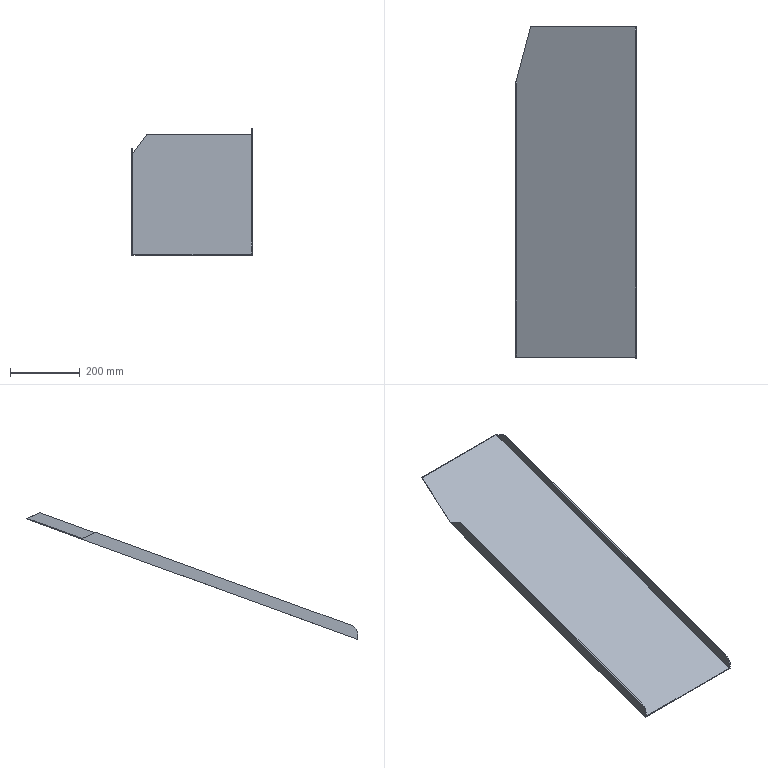Part | NX | features solid 2 | 1 solid | 14 faces | box 344.217 x 951.809 x 363.702 mm | volume 792307 mm3 | plane 12 | cylinder 2 | commonest cylinder face diameters 60 x2
STEP:
#1=CARTESIAN_POINT('',(718.,-1180.,-590.79));
#2=VERTEX_POINT('',#1);
#3=CARTESIAN_POINT('',(375.783,-1180.,-590.79));
#4=VERTEX_POINT('',#3);
#5=CARTESIAN_POINT('',(-625.,-1180.,-590.79));
#6=DIRECTION('',(1.,0.,0.));
#7=VECTOR('',#6,1000.);
#8=LINE('',#5,#7);
#9=EDGE_CURVE('',#2,#4,#8,.F.);
#10=ORIENTED_EDGE('',*,*,#9,.F.);
#11=CARTESIAN_POINT('',(718.,-1180.,-588.662));
#12=VERTEX_POINT('',#11);
#13=CARTESIAN_POINT('',(718.,-1180.,-730.));
#14=DIRECTION('',(0.,0.,-1.));
#15=VECTOR('',#14,1000.);
#16=LINE('',#13,#15);
#17=EDGE_CURVE('',#2,#12,#16,.F.);
#18=ORIENTED_EDGE('',*,*,#17,.T.);
#19=CARTESIAN_POINT('',(377.783,-1180.,-588.662));
#20=VERTEX_POINT('',#19);
#21=CARTESIAN_POINT('',(-625.,-1180.,-588.662));
#22=DIRECTION('',(1.,0.,0.));
#23=VECTOR('',#22,1000.);
#24=LINE('',#21,#23);
#25=EDGE_CURVE('',#12,#20,#24,.F.);
#26=ORIENTED_EDGE('',*,*,#25,.T.);
#27=CARTESIAN_POINT('',(375.783,-1180.,-588.662));
#28=VERTEX_POINT('',#27);
#29=CARTESIAN_POINT('',(375.783,-1180.,-588.662));
#30=DIRECTION('',(1.,0.,0.));
#31=VECTOR('',#30,1000.);
#32=LINE('',#29,#31);
#33=EDGE_CURVE('',#28,#20,#32,.T.);
#34=ORIENTED_EDGE('',*,*,#33,.F.);
#35=CARTESIAN_POINT('',(375.783,-1180.,-730.));
#36=DIRECTION('',(0.,0.,1.));
#37=VECTOR('',#36,1000.);
#38=LINE('',#35,#37);
#39=EDGE_CURVE('',#28,#4,#38,.F.);
#40=ORIENTED_EDGE('',*,*,#39,.T.);
#41=EDGE_LOOP('',(#10,#18,#26,#34,#40));
#42=FACE_BOUND('',#41,.T.);
#43=CARTESIAN_POINT('',(-625.,-1180.,-730.));
#44=DIRECTION('',(0.,1.,0.));
#45=DIRECTION('',(1.,0.,0.));
#46=AXIS2_PLACEMENT_3D('',#43,#44,#45);
#47=PLANE('',#46);
#48=ADVANCED_FACE('',(#42),#47,.F.);
#49=CARTESIAN_POINT('',(718.,-232.563,-243.823));
#50=VERTEX_POINT('',#49);
#51=CARTESIAN_POINT('',(718.,-1653.904,-761.149));
#52=DIRECTION('',(0.,0.9397,0.342));
#53=VECTOR('',#52,1000.);
#54=LINE('',#51,#53);
#55=EDGE_CURVE('',#12,#50,#54,.T.);
#56=ORIENTED_EDGE('',*,*,#55,.T.);
#57=CARTESIAN_POINT('',(418.101,-232.563,-243.823));
#58=VERTEX_POINT('',#57);
#59=CARTESIAN_POINT('',(620.,-232.563,-243.823));
#60=DIRECTION('',(-1.,0.,0.));
#61=VECTOR('',#60,1000.);
#62=LINE('',#59,#61);
#63=EDGE_CURVE('',#50,#58,#62,.T.);
#64=ORIENTED_EDGE('',*,*,#63,.T.);
#65=CARTESIAN_POINT('',(375.783,-390.494,-301.305));
#66=VERTEX_POINT('',#65);
#67=CARTESIAN_POINT('',(71.996,-1524.243,-713.956));
#68=DIRECTION('',(-0.2442,-0.9113,-0.3317));
#69=VECTOR('',#68,1000.);
#70=LINE('',#67,#69);
#71=EDGE_CURVE('',#58,#66,#70,.T.);
#72=ORIENTED_EDGE('',*,*,#71,.T.);
#73=CARTESIAN_POINT('',(377.783,-390.494,-301.305));
#74=VERTEX_POINT('',#73);
#75=CARTESIAN_POINT('',(375.783,-390.494,-301.305));
#76=DIRECTION('',(1.,0.,0.));
#77=VECTOR('',#76,1000.);
#78=LINE('',#75,#77);
#79=EDGE_CURVE('',#66,#74,#78,.T.);
#80=ORIENTED_EDGE('',*,*,#79,.T.);
#81=CARTESIAN_POINT('',(377.783,-1180.,-588.662));
#82=DIRECTION('',(0.,0.9397,0.342));
#83=VECTOR('',#82,1000.);
#84=LINE('',#81,#83);
#85=EDGE_CURVE('',#20,#74,#84,.T.);
#86=ORIENTED_EDGE('',*,*,#85,.F.);
#87=ORIENTED_EDGE('',*,*,#25,.F.);
#88=EDGE_LOOP('',(#56,#64,#72,#80,#86,#87));
#89=FACE_BOUND('',#88,.T.);
#90=CARTESIAN_POINT('',(620.,-1653.904,-761.149));
#91=DIRECTION('',(0.,-0.342,0.9397));
#92=DIRECTION('',(1.,0.,0.));
#93=AXIS2_PLACEMENT_3D('',#90,#91,#92);
#94=PLANE('',#93);
#95=ADVANCED_FACE('',(#89),#94,.T.);
#96=ORIENTED_EDGE('',*,*,#71,.F.);
#97=CARTESIAN_POINT('',(418.604,-230.,-245.018));
#98=VERTEX_POINT('',#97);
#99=CARTESIAN_POINT('',(420.543,-220.131,-249.621));
#100=DIRECTION('',(0.1753,0.8923,-0.4161));
#101=VECTOR('',#100,1000.);
#102=LINE('',#99,#101);
#103=EDGE_CURVE('',#58,#98,#102,.T.);
#104=ORIENTED_EDGE('',*,*,#103,.T.);
#105=CARTESIAN_POINT('',(375.783,-389.81,-303.185));
#106=VERTEX_POINT('',#105);
#107=CARTESIAN_POINT('',(71.996,-1523.559,-715.835));
#108=DIRECTION('',(-0.2442,-0.9113,-0.3317));
#109=VECTOR('',#108,1000.);
#110=LINE('',#107,#109);
#111=EDGE_CURVE('',#98,#106,#110,.T.);
#112=ORIENTED_EDGE('',*,*,#111,.T.);
#113=CARTESIAN_POINT('',(375.783,-390.494,-301.305));
#114=DIRECTION('',(0.,0.342,-0.9397));
#115=VECTOR('',#114,1000.);
#116=LINE('',#113,#115);
#117=EDGE_CURVE('',#66,#106,#116,.T.);
#118=ORIENTED_EDGE('',*,*,#117,.F.);
#119=EDGE_LOOP('',(#96,#104,#112,#118));
#120=FACE_BOUND('',#119,.T.);
#121=CARTESIAN_POINT('',(71.996,-1524.243,-713.956));
#122=DIRECTION('',(0.9697,-0.2294,-0.08351));
#123=DIRECTION('',(0.2302,0.9731,0.));
#124=AXIS2_PLACEMENT_3D('',#121,#122,#123);
#125=PLANE('',#124);
#126=ADVANCED_FACE('',(#120),#125,.F.);
#127=CARTESIAN_POINT('',(375.783,-1162.07,-550.21));
#128=VERTEX_POINT('',#127);
#129=CARTESIAN_POINT('',(375.783,-428.946,-283.375));
#130=VERTEX_POINT('',#129);
#131=CARTESIAN_POINT('',(375.783,-1190.261,-560.471));
#132=DIRECTION('',(0.,0.9397,0.342));
#133=VECTOR('',#132,1000.);
#134=LINE('',#131,#133);
#135=EDGE_CURVE('',#128,#130,#134,.T.);
#136=ORIENTED_EDGE('',*,*,#135,.T.);
#137=CARTESIAN_POINT('',(375.783,-1252.121,100.478));
#138=DIRECTION('',(0.,0.9063,-0.4226));
#139=VECTOR('',#138,1000.);
#140=LINE('',#137,#139);
#141=EDGE_CURVE('',#130,#66,#140,.T.);
#142=ORIENTED_EDGE('',*,*,#141,.T.);
#143=ORIENTED_EDGE('',*,*,#117,.T.);
#144=CARTESIAN_POINT('',(375.783,-1653.22,-763.028));
#145=DIRECTION('',(0.,0.9397,0.342));
#146=VECTOR('',#145,1000.);
#147=LINE('',#144,#146);
#148=EDGE_CURVE('',#4,#106,#147,.T.);
#149=ORIENTED_EDGE('',*,*,#148,.F.);
#150=ORIENTED_EDGE('',*,*,#39,.F.);
#151=CARTESIAN_POINT('',(375.783,-1151.809,-578.401));
#152=DIRECTION('',(1.,0.,0.));
#153=DIRECTION('',(0.,1.,0.));
#154=AXIS2_PLACEMENT_3D('',#151,#152,#153);
#155=CIRCLE('',#154,30.);
#156=EDGE_CURVE('',#28,#128,#155,.F.);
#157=ORIENTED_EDGE('',*,*,#156,.T.);
#158=EDGE_LOOP('',(#136,#142,#143,#149,#150,#157));
#159=FACE_BOUND('',#158,.T.);
#160=CARTESIAN_POINT('',(375.783,-1653.904,-761.149));
#161=DIRECTION('',(-1.,0.,0.));
#162=DIRECTION('',(0.,-1.,0.));
#163=AXIS2_PLACEMENT_3D('',#160,#161,#162);
#164=PLANE('',#163);
#165=ADVANCED_FACE('',(#159),#164,.T.);
#166=CARTESIAN_POINT('',(720.,-1180.,-590.79));
#167=VERTEX_POINT('',#166);
#168=CARTESIAN_POINT('',(720.,-230.,-245.018));
#169=VERTEX_POINT('',#168);
#170=CARTESIAN_POINT('',(720.,-1653.22,-763.028));
#171=DIRECTION('',(0.,0.9397,0.342));
#172=VECTOR('',#171,1000.);
#173=LINE('',#170,#172);
#174=EDGE_CURVE('',#167,#169,#173,.T.);
#175=ORIENTED_EDGE('',*,*,#174,.T.);
#176=CARTESIAN_POINT('',(720.,-268.451,-227.088));
#177=VERTEX_POINT('',#176);
#178=CARTESIAN_POINT('',(720.,-268.451,-227.088));
#179=DIRECTION('',(0.,-0.9063,0.4226));
#180=VECTOR('',#179,1000.);
#181=LINE('',#178,#180);
#182=EDGE_CURVE('',#169,#177,#181,.T.);
#183=ORIENTED_EDGE('',*,*,#182,.T.);
#184=CARTESIAN_POINT('',(720.,-1162.07,-552.339));
#185=VERTEX_POINT('',#184);
#186=CARTESIAN_POINT('',(720.,-1190.261,-562.599));
#187=DIRECTION('',(0.,0.9397,0.342));
#188=VECTOR('',#187,1000.);
#189=LINE('',#186,#188);
#190=EDGE_CURVE('',#185,#177,#189,.T.);
#191=ORIENTED_EDGE('',*,*,#190,.F.);
#192=CARTESIAN_POINT('',(720.,-1151.809,-580.529));
#193=DIRECTION('',(1.,0.,0.));
#194=DIRECTION('',(0.,0.,-1.));
#195=AXIS2_PLACEMENT_3D('',#192,#193,#194);
#196=CIRCLE('',#195,30.);
#197=EDGE_CURVE('',#185,#167,#196,.T.);
#198=ORIENTED_EDGE('',*,*,#197,.T.);
#199=EDGE_LOOP('',(#175,#183,#191,#198));
#200=FACE_BOUND('',#199,.T.);
#201=CARTESIAN_POINT('',(720.,-1653.904,-761.149));
#202=DIRECTION('',(-1.,0.,0.));
#203=DIRECTION('',(0.,0.,1.));
#204=AXIS2_PLACEMENT_3D('',#201,#202,#203);
#205=PLANE('',#204);
#206=ADVANCED_FACE('',(#200),#205,.F.);
#207=CARTESIAN_POINT('',(-625.,-1180.,-590.79));
#208=DIRECTION('',(1.,0.,0.));
#209=VECTOR('',#208,1000.);
#210=LINE('',#207,#209);
#211=EDGE_CURVE('',#167,#2,#210,.F.);
#212=ORIENTED_EDGE('',*,*,#211,.T.);
#213=ORIENTED_EDGE('',*,*,#9,.T.);
#214=ORIENTED_EDGE('',*,*,#148,.T.);
#215=ORIENTED_EDGE('',*,*,#111,.F.);
#216=CARTESIAN_POINT('',(620.,-230.,-245.018));
#217=DIRECTION('',(1.,0.,0.));
#218=VECTOR('',#217,1000.);
#219=LINE('',#216,#218);
#220=EDGE_CURVE('',#98,#169,#219,.T.);
#221=ORIENTED_EDGE('',*,*,#220,.T.);
#222=ORIENTED_EDGE('',*,*,#174,.F.);
#223=EDGE_LOOP('',(#212,#213,#214,#215,#221,#222));
#224=FACE_BOUND('',#223,.T.);
#225=CARTESIAN_POINT('',(620.,-1653.22,-763.028));
#226=DIRECTION('',(0.,-0.342,0.9397));
#227=DIRECTION('',(1.,0.,0.));
#228=AXIS2_PLACEMENT_3D('',#225,#226,#227);
#229=PLANE('',#228);
#230=ADVANCED_FACE('',(#224),#229,.F.);
#231=ORIENTED_EDGE('',*,*,#190,.T.);
#232=CARTESIAN_POINT('',(718.,-268.451,-227.088));
#233=VERTEX_POINT('',#232);
#234=CARTESIAN_POINT('',(718.,-268.451,-227.088));
#235=DIRECTION('',(-1.,0.,0.));
#236=VECTOR('',#235,1000.);
#237=LINE('',#234,#236);
#238=EDGE_CURVE('',#177,#233,#237,.T.);
#239=ORIENTED_EDGE('',*,*,#238,.T.);
#240=CARTESIAN_POINT('',(718.,-1162.07,-552.339));
#241=VERTEX_POINT('',#240);
#242=CARTESIAN_POINT('',(718.,-1190.261,-562.599));
#243=DIRECTION('',(0.,0.9397,0.342));
#244=VECTOR('',#243,1000.);
#245=LINE('',#242,#244);
#246=EDGE_CURVE('',#241,#233,#245,.T.);
#247=ORIENTED_EDGE('',*,*,#246,.F.);
#248=CARTESIAN_POINT('',(720.,-1162.07,-552.339));
#249=DIRECTION('',(-1.,0.,0.));
#250=VECTOR('',#249,1000.);
#251=LINE('',#248,#250);
#252=EDGE_CURVE('',#241,#185,#251,.F.);
#253=ORIENTED_EDGE('',*,*,#252,.T.);
#254=EDGE_LOOP('',(#231,#239,#247,#253));
#255=FACE_BOUND('',#254,.T.);
#256=CARTESIAN_POINT('',(720.,-1190.261,-562.599));
#257=DIRECTION('',(0.,0.342,-0.9397));
#258=DIRECTION('',(0.,0.9397,0.342));
#259=AXIS2_PLACEMENT_3D('',#256,#257,#258);
#260=PLANE('',#259);
#261=ADVANCED_FACE('',(#255),#260,.F.);
#262=ORIENTED_EDGE('',*,*,#246,.T.);
#263=CARTESIAN_POINT('',(718.,-268.451,-227.088));
#264=DIRECTION('',(0.,0.9063,-0.4226));
#265=VECTOR('',#264,1000.);
#266=LINE('',#263,#265);
#267=EDGE_CURVE('',#233,#50,#266,.T.);
#268=ORIENTED_EDGE('',*,*,#267,.T.);
#269=ORIENTED_EDGE('',*,*,#55,.F.);
#270=ORIENTED_EDGE('',*,*,#17,.F.);
#271=CARTESIAN_POINT('',(718.,-1151.809,-580.529));
#272=DIRECTION('',(1.,0.,0.));
#273=DIRECTION('',(0.,0.,-1.));
#274=AXIS2_PLACEMENT_3D('',#271,#272,#273);
#275=CIRCLE('',#274,30.);
#276=EDGE_CURVE('',#2,#241,#275,.F.);
#277=ORIENTED_EDGE('',*,*,#276,.T.);
#278=EDGE_LOOP('',(#262,#268,#269,#270,#277));
#279=FACE_BOUND('',#278,.T.);
#280=CARTESIAN_POINT('',(718.,-1180.,-590.79));
#281=DIRECTION('',(1.,0.,0.));
#282=DIRECTION('',(0.,0.,-1.));
#283=AXIS2_PLACEMENT_3D('',#280,#281,#282);
#284=PLANE('',#283);
#285=ADVANCED_FACE('',(#279),#284,.F.);
#286=ORIENTED_EDGE('',*,*,#197,.F.);
#287=ORIENTED_EDGE('',*,*,#252,.F.);
#288=ORIENTED_EDGE('',*,*,#276,.F.);
#289=ORIENTED_EDGE('',*,*,#211,.F.);
#290=EDGE_LOOP('',(#286,#287,#288,#289));
#291=FACE_BOUND('',#290,.T.);
#292=CARTESIAN_POINT('',(720.,-1151.809,-580.529));
#293=DIRECTION('',(-1.,0.,0.));
#294=DIRECTION('',(0.,0.,1.));
#295=AXIS2_PLACEMENT_3D('',#292,#293,#294);
#296=CYLINDRICAL_SURFACE('',#295,30.);
#297=ADVANCED_FACE('',(#291),#296,.T.);
#298=CARTESIAN_POINT('',(377.783,-1162.07,-550.21));
#299=VERTEX_POINT('',#298);
#300=CARTESIAN_POINT('',(377.783,-428.946,-283.375));
#301=VERTEX_POINT('',#300);
#302=CARTESIAN_POINT('',(377.783,-1190.261,-560.471));
#303=DIRECTION('',(0.,0.9397,0.342));
#304=VECTOR('',#303,1000.);
#305=LINE('',#302,#304);
#306=EDGE_CURVE('',#299,#301,#305,.T.);
#307=ORIENTED_EDGE('',*,*,#306,.T.);
#308=CARTESIAN_POINT('',(375.783,-428.946,-283.375));
#309=DIRECTION('',(1.,0.,0.));
#310=VECTOR('',#309,1000.);
#311=LINE('',#308,#310);
#312=EDGE_CURVE('',#301,#130,#311,.F.);
#313=ORIENTED_EDGE('',*,*,#312,.T.);
#314=ORIENTED_EDGE('',*,*,#135,.F.);
#315=CARTESIAN_POINT('',(375.783,-1162.07,-550.21));
#316=DIRECTION('',(-1.,0.,0.));
#317=VECTOR('',#316,1000.);
#318=LINE('',#315,#317);
#319=EDGE_CURVE('',#128,#299,#318,.F.);
#320=ORIENTED_EDGE('',*,*,#319,.T.);
#321=EDGE_LOOP('',(#307,#313,#314,#320));
#322=FACE_BOUND('',#321,.T.);
#323=CARTESIAN_POINT('',(375.783,-1190.261,-560.471));
#324=DIRECTION('',(0.,0.342,-0.9397));
#325=DIRECTION('',(0.,0.9397,0.342));
#326=AXIS2_PLACEMENT_3D('',#323,#324,#325);
#327=PLANE('',#326);
#328=ADVANCED_FACE('',(#322),#327,.F.);
#329=ORIENTED_EDGE('',*,*,#85,.T.);
#330=CARTESIAN_POINT('',(377.783,-928.925,-50.231));
#331=DIRECTION('',(0.,-0.9063,0.4226));
#332=VECTOR('',#331,1000.);
#333=LINE('',#330,#332);
#334=EDGE_CURVE('',#74,#301,#333,.T.);
#335=ORIENTED_EDGE('',*,*,#334,.T.);
#336=ORIENTED_EDGE('',*,*,#306,.F.);
#337=CARTESIAN_POINT('',(377.783,-1151.809,-578.401));
#338=DIRECTION('',(1.,0.,0.));
#339=DIRECTION('',(0.,1.,0.));
#340=AXIS2_PLACEMENT_3D('',#337,#338,#339);
#341=CIRCLE('',#340,30.);
#342=EDGE_CURVE('',#299,#20,#341,.T.);
#343=ORIENTED_EDGE('',*,*,#342,.T.);
#344=EDGE_LOOP('',(#329,#335,#336,#343));
#345=FACE_BOUND('',#344,.T.);
#346=CARTESIAN_POINT('',(377.783,-1180.,-588.662));
#347=DIRECTION('',(1.,0.,0.));
#348=DIRECTION('',(0.,1.,0.));
#349=AXIS2_PLACEMENT_3D('',#346,#347,#348);
#350=PLANE('',#349);
#351=ADVANCED_FACE('',(#345),#350,.T.);
#352=ORIENTED_EDGE('',*,*,#156,.F.);
#353=ORIENTED_EDGE('',*,*,#33,.T.);
#354=ORIENTED_EDGE('',*,*,#342,.F.);
#355=ORIENTED_EDGE('',*,*,#319,.F.);
#356=EDGE_LOOP('',(#352,#353,#354,#355));
#357=FACE_BOUND('',#356,.T.);
#358=CARTESIAN_POINT('',(375.783,-1151.809,-578.401));
#359=DIRECTION('',(1.,0.,0.));
#360=DIRECTION('',(0.,1.,0.));
#361=AXIS2_PLACEMENT_3D('',#358,#359,#360);
#362=CYLINDRICAL_SURFACE('',#361,30.);
#363=ADVANCED_FACE('',(#357),#362,.T.);
#364=ORIENTED_EDGE('',*,*,#141,.F.);
#365=ORIENTED_EDGE('',*,*,#312,.F.);
#366=ORIENTED_EDGE('',*,*,#334,.F.);
#367=ORIENTED_EDGE('',*,*,#79,.F.);
#368=EDGE_LOOP('',(#364,#365,#366,#367));
#369=FACE_BOUND('',#368,.T.);
#370=CARTESIAN_POINT('',(375.783,-390.494,-301.305));
#371=DIRECTION('',(0.,0.4226,0.9063));
#372=DIRECTION('',(0.,-0.9063,0.4226));
#373=AXIS2_PLACEMENT_3D('',#370,#371,#372);
#374=PLANE('',#373);
#375=ADVANCED_FACE('',(#369),#374,.T.);
#376=ORIENTED_EDGE('',*,*,#182,.F.);
#377=ORIENTED_EDGE('',*,*,#220,.F.);
#378=ORIENTED_EDGE('',*,*,#103,.F.);
#379=ORIENTED_EDGE('',*,*,#63,.F.);
#380=ORIENTED_EDGE('',*,*,#267,.F.);
#381=ORIENTED_EDGE('',*,*,#238,.F.);
#382=EDGE_LOOP('',(#376,#377,#378,#379,#380,#381));
#383=FACE_BOUND('',#382,.T.);
#384=CARTESIAN_POINT('',(720.,-268.451,-227.088));
#385=DIRECTION('',(0.,0.4226,0.9063));
#386=DIRECTION('',(0.,-0.9063,0.4226));
#387=AXIS2_PLACEMENT_3D('',#384,#385,#386);
#388=PLANE('',#387);
#389=ADVANCED_FACE('',(#383),#388,.T.);
#390=CLOSED_SHELL('',(#48,#95,#126,#165,#206,#230,#261,#285,#297,#328,#351,#363,#375,#389));
#391=MANIFOLD_SOLID_BREP('',#390);
#392=(LENGTH_UNIT()NAMED_UNIT(*)SI_UNIT(.MILLI.,.METRE.));
#393=UNCERTAINTY_MEASURE_WITH_UNIT(LENGTH_MEASURE(0.00001),#392,'','');
#394=(NAMED_UNIT(*)PLANE_ANGLE_UNIT()SI_UNIT($,.RADIAN.));
#395=(NAMED_UNIT(*)SI_UNIT($,.STERADIAN.)SOLID_ANGLE_UNIT());
#396=(GEOMETRIC_REPRESENTATION_CONTEXT(3)GLOBAL_UNCERTAINTY_ASSIGNED_CONTEXT((#393))GLOBAL_UNIT_ASSIGNED_CONTEXT((#392,#394,#395))REPRESENTATION_CONTEXT('',''));
#397=ADVANCED_BREP_SHAPE_REPRESENTATION('',(#391),#396);